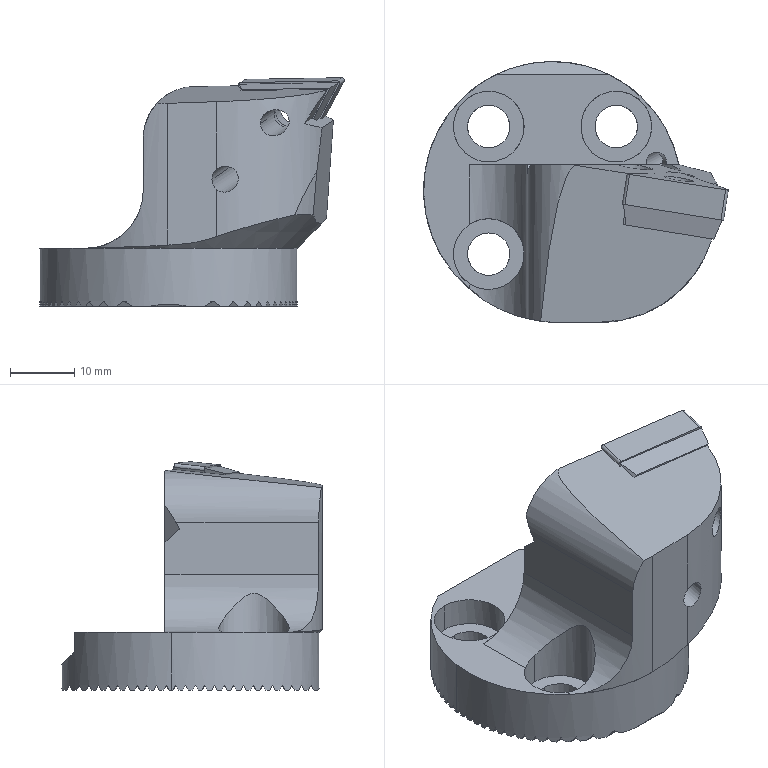NC program | Mastercam | posted with a generic post
Whole program:
%
:0001()
(MATERIAL - ALUMINUM MM - 2024)
(T7|4 FEMF |H7|D7|WEAR COMP|TOOL DIA. - 4.|XY STOCK TO LEAVE - 0.|Z STOCK TO LEAVE - -.05)
N100 G21
N102 G0 G17 G40 G80 G90 G94 G98
N104 G0 G28 G91 Z0.
N106 G0 G28 X0. Y0.
(4 FEMF |TOOL - 7|DIA. OFF. - 7|LEN. - 7|TOOL DIA. - 4.)
N108 T7 M6
N110 G0 G54 G90 X30.972 Y22.875 C8.409 B-83.617 S3500 M3
N112 G43 H7 Z61.427
N114 Z12.427
N116 G1 Z3.077 F2000.
N118 G41 D7 X29.834 Y22.246 F400.
N120 X25.131 Y19.646
N122 G40 X24.606 Y19.356
N124 G0 Z53.077
N126 X30.972 Y22.875
N128 Z12.427
N130 G1 Z3.077 F2000.
N132 G41 D7 X29.834 Y22.246 F400.
N134 X25.131 Y19.646
N136 G40 X24.606 Y19.356
N138 G0 Z61.427
N140 Z61.82
N142 X24.384 Y19.111
N144 C9.578 B-83.596
N146 Z12.82
N148 G1 Z3.47 F2000.
N150 G41 D7 X25.07 Y18.7 F400.
N152 X34.588 Y12.995
N154 G40 X36.303 Y11.967
N156 G0 Z53.47
N158 X24.384 Y19.111
N160 Z12.82
N162 G1 Z3.47 F2000.
N164 G41 D7 X25.07 Y18.7 F400.
N166 X34.588 Y12.995
N168 G40 X36.303 Y11.967
N170 G0 Z61.82
N172 M5
N174 G0 G28 G91 Z0.
N176 G0 G28 X0. Y0.
N178 G28 C0. B0.
N180 M30
%